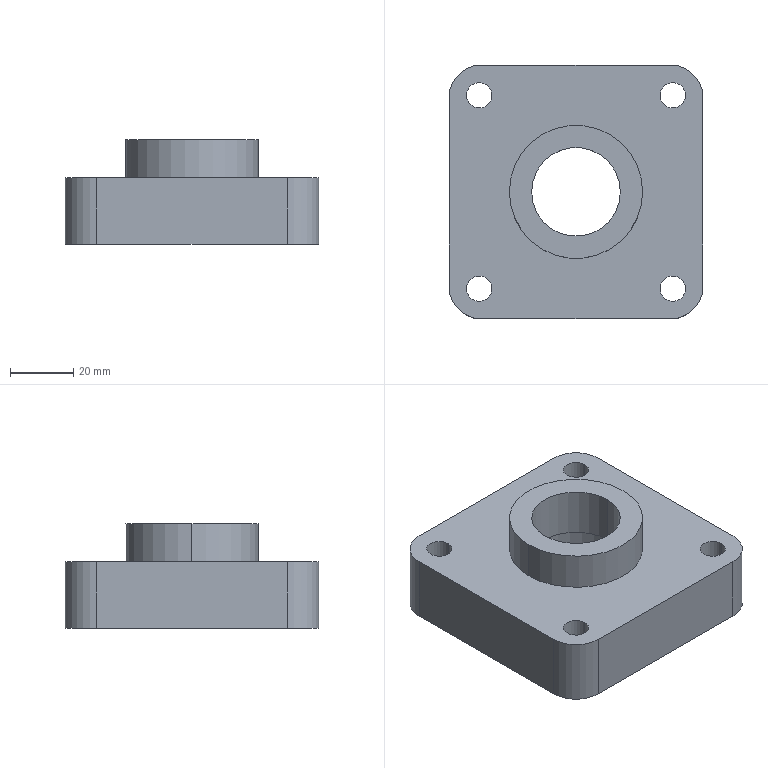Part | SolidWorks | features Fillet 3, ICE 2, MirrorPattern 2, Extrusion 1, RevCut 1 | 1 solid | 39 faces | box 80 x 80 x 33 mm | volume 110292 mm3 | cylinder 24 | plane 11 | torus 4 | commonest cylinder face diameters 8 x8 20 x4 28 x2 35 x2 40 x2 42 x2
STEP:
#1=CARTESIAN_POINT('',(19.,0.,17.5));
#2=VERTEX_POINT('',#1);
#3=CARTESIAN_POINT('',(-19.,0.,17.5));
#4=VERTEX_POINT('',#3);
#5=CARTESIAN_POINT('',(0.,0.,17.5));
#6=DIRECTION('',(0.,0.,-1.));
#7=DIRECTION('',(-1.,0.,0.));
#8=AXIS2_PLACEMENT_3D('',#5,#6,#7);
#9=CIRCLE('',#8,19.);
#10=EDGE_CURVE('',#2,#4,#9,.T.);
#11=ORIENTED_EDGE('',*,*,#10,.F.);
#12=CARTESIAN_POINT('',(20.,0.,16.5));
#13=VERTEX_POINT('',#12);
#14=CARTESIAN_POINT('',(19.,0.,16.5));
#15=DIRECTION('',(0.,1.,0.));
#16=DIRECTION('',(-1.,0.,0.));
#17=AXIS2_PLACEMENT_3D('',#14,#15,#16);
#18=CIRCLE('',#17,1.);
#19=EDGE_CURVE('',#2,#13,#18,.T.);
#20=ORIENTED_EDGE('',*,*,#19,.T.);
#21=CARTESIAN_POINT('',(-20.,0.,16.5));
#22=VERTEX_POINT('',#21);
#23=CARTESIAN_POINT('',(0.,0.,16.5));
#24=DIRECTION('',(0.,0.,1.));
#25=DIRECTION('',(-1.,0.,0.));
#26=AXIS2_PLACEMENT_3D('',#23,#24,#25);
#27=CIRCLE('',#26,20.);
#28=EDGE_CURVE('',#22,#13,#27,.T.);
#29=ORIENTED_EDGE('',*,*,#28,.F.);
#30=CARTESIAN_POINT('',(-19.,0.,16.5));
#31=DIRECTION('',(0.,-1.,0.));
#32=DIRECTION('',(0.,0.,-1.));
#33=AXIS2_PLACEMENT_3D('',#30,#31,#32);
#34=CIRCLE('',#33,1.);
#35=EDGE_CURVE('',#4,#22,#34,.T.);
#36=ORIENTED_EDGE('',*,*,#35,.F.);
#37=EDGE_LOOP('',(#11,#20,#29,#36));
#38=FACE_OUTER_BOUND('',#37,.T.);
#39=CARTESIAN_POINT('',(0.,0.,16.5));
#40=DIRECTION('',(0.,0.,-1.));
#41=DIRECTION('',(-1.,0.,0.));
#42=AXIS2_PLACEMENT_3D('',#39,#40,#41);
#43=TOROIDAL_SURFACE('',#42,19.,1.);
#44=ADVANCED_FACE('',(#38),#43,.F.);
#45=CARTESIAN_POINT('',(29.,0.,2.5));
#46=VERTEX_POINT('',#45);
#47=CARTESIAN_POINT('',(-29.,0.,2.5));
#48=VERTEX_POINT('',#47);
#49=CARTESIAN_POINT('',(0.,0.,2.5));
#50=DIRECTION('',(0.,0.,-1.));
#51=DIRECTION('',(-1.,0.,0.));
#52=AXIS2_PLACEMENT_3D('',#49,#50,#51);
#53=CIRCLE('',#52,29.);
#54=EDGE_CURVE('',#46,#48,#53,.T.);
#55=ORIENTED_EDGE('',*,*,#54,.F.);
#56=CARTESIAN_POINT('',(30.,0.,1.5));
#57=VERTEX_POINT('',#56);
#58=CARTESIAN_POINT('',(29.,0.,1.5));
#59=DIRECTION('',(0.,1.,0.));
#60=DIRECTION('',(-1.,0.,0.));
#61=AXIS2_PLACEMENT_3D('',#58,#59,#60);
#62=CIRCLE('',#61,1.);
#63=EDGE_CURVE('',#46,#57,#62,.T.);
#64=ORIENTED_EDGE('',*,*,#63,.T.);
#65=CARTESIAN_POINT('',(-30.,0.,1.5));
#66=VERTEX_POINT('',#65);
#67=CARTESIAN_POINT('',(0.,0.,1.5));
#68=DIRECTION('',(0.,0.,1.));
#69=DIRECTION('',(-1.,0.,0.));
#70=AXIS2_PLACEMENT_3D('',#67,#68,#69);
#71=CIRCLE('',#70,30.);
#72=EDGE_CURVE('',#66,#57,#71,.T.);
#73=ORIENTED_EDGE('',*,*,#72,.F.);
#74=CARTESIAN_POINT('',(-29.,0.,1.5));
#75=DIRECTION('',(0.,-1.,0.));
#76=DIRECTION('',(0.,0.,-1.));
#77=AXIS2_PLACEMENT_3D('',#74,#75,#76);
#78=CIRCLE('',#77,1.);
#79=EDGE_CURVE('',#48,#66,#78,.T.);
#80=ORIENTED_EDGE('',*,*,#79,.F.);
#81=EDGE_LOOP('',(#55,#64,#73,#80));
#82=FACE_OUTER_BOUND('',#81,.T.);
#83=CARTESIAN_POINT('',(0.,0.,1.5));
#84=DIRECTION('',(0.,0.,-1.));
#85=DIRECTION('',(-1.,0.,0.));
#86=AXIS2_PLACEMENT_3D('',#83,#84,#85);
#87=TOROIDAL_SURFACE('',#86,29.,1.);
#88=ADVANCED_FACE('',(#82),#87,.F.);
#89=CARTESIAN_POINT('',(34.5,30.5,0.));
#90=VERTEX_POINT('',#89);
#91=CARTESIAN_POINT('',(26.5,30.5,0.));
#92=VERTEX_POINT('',#91);
#93=CARTESIAN_POINT('',(30.5,30.5,0.));
#94=DIRECTION('',(0.,0.,-1.));
#95=DIRECTION('',(-1.,0.,0.));
#96=AXIS2_PLACEMENT_3D('',#93,#94,#95);
#97=CIRCLE('',#96,4.);
#98=EDGE_CURVE('',#90,#92,#97,.T.);
#99=ORIENTED_EDGE('',*,*,#98,.T.);
#100=CARTESIAN_POINT('',(26.5,30.5,21.));
#101=VERTEX_POINT('',#100);
#102=CARTESIAN_POINT('',(26.5,30.5,0.));
#103=DIRECTION('',(0.,0.,1.));
#104=VECTOR('',#103,1000.);
#105=LINE('',#102,#104);
#106=EDGE_CURVE('',#92,#101,#105,.T.);
#107=ORIENTED_EDGE('',*,*,#106,.T.);
#108=CARTESIAN_POINT('',(34.5,30.5,21.));
#109=VERTEX_POINT('',#108);
#110=CARTESIAN_POINT('',(30.5,30.5,21.));
#111=DIRECTION('',(0.,0.,-1.));
#112=DIRECTION('',(-1.,0.,0.));
#113=AXIS2_PLACEMENT_3D('',#110,#111,#112);
#114=CIRCLE('',#113,4.);
#115=EDGE_CURVE('',#109,#101,#114,.T.);
#116=ORIENTED_EDGE('',*,*,#115,.F.);
#117=CARTESIAN_POINT('',(34.5,30.5,0.));
#118=DIRECTION('',(0.,0.,1.));
#119=VECTOR('',#118,1000.);
#120=LINE('',#117,#119);
#121=EDGE_CURVE('',#90,#109,#120,.T.);
#122=ORIENTED_EDGE('',*,*,#121,.F.);
#123=EDGE_LOOP('',(#99,#107,#116,#122));
#124=FACE_OUTER_BOUND('',#123,.T.);
#125=CARTESIAN_POINT('',(30.5,30.5,0.));
#126=DIRECTION('',(0.,0.,1.));
#127=DIRECTION('',(1.,0.,0.));
#128=AXIS2_PLACEMENT_3D('',#125,#126,#127);
#129=CYLINDRICAL_SURFACE('',#128,4.);
#130=ADVANCED_FACE('',(#124),#129,.F.);
#131=CARTESIAN_POINT('',(26.5,-30.5,0.));
#132=VERTEX_POINT('',#131);
#133=CARTESIAN_POINT('',(34.5,-30.5,0.));
#134=VERTEX_POINT('',#133);
#135=CARTESIAN_POINT('',(30.5,-30.5,0.));
#136=DIRECTION('',(0.,0.,1.));
#137=DIRECTION('',(-1.,0.,0.));
#138=AXIS2_PLACEMENT_3D('',#135,#136,#137);
#139=CIRCLE('',#138,4.);
#140=EDGE_CURVE('',#132,#134,#139,.T.);
#141=ORIENTED_EDGE('',*,*,#140,.F.);
#142=CARTESIAN_POINT('',(26.5,-30.5,21.));
#143=VERTEX_POINT('',#142);
#144=CARTESIAN_POINT('',(26.5,-30.5,0.));
#145=DIRECTION('',(0.,0.,1.));
#146=VECTOR('',#145,1000.);
#147=LINE('',#144,#146);
#148=EDGE_CURVE('',#132,#143,#147,.T.);
#149=ORIENTED_EDGE('',*,*,#148,.T.);
#150=CARTESIAN_POINT('',(34.5,-30.5,21.));
#151=VERTEX_POINT('',#150);
#152=CARTESIAN_POINT('',(30.5,-30.5,21.));
#153=DIRECTION('',(0.,0.,1.));
#154=DIRECTION('',(-1.,0.,0.));
#155=AXIS2_PLACEMENT_3D('',#152,#153,#154);
#156=CIRCLE('',#155,4.);
#157=EDGE_CURVE('',#143,#151,#156,.T.);
#158=ORIENTED_EDGE('',*,*,#157,.T.);
#159=CARTESIAN_POINT('',(34.5,-30.5,0.));
#160=DIRECTION('',(0.,0.,1.));
#161=VECTOR('',#160,1000.);
#162=LINE('',#159,#161);
#163=EDGE_CURVE('',#134,#151,#162,.T.);
#164=ORIENTED_EDGE('',*,*,#163,.F.);
#165=EDGE_LOOP('',(#141,#149,#158,#164));
#166=FACE_OUTER_BOUND('',#165,.T.);
#167=CARTESIAN_POINT('',(30.5,-30.5,0.));
#168=DIRECTION('',(0.,0.,1.));
#169=DIRECTION('',(1.,0.,0.));
#170=AXIS2_PLACEMENT_3D('',#167,#168,#169);
#171=CYLINDRICAL_SURFACE('',#170,4.);
#172=ADVANCED_FACE('',(#166),#171,.F.);
#173=CARTESIAN_POINT('',(-26.5,-30.5,0.));
#174=VERTEX_POINT('',#173);
#175=CARTESIAN_POINT('',(-34.5,-30.5,0.));
#176=VERTEX_POINT('',#175);
#177=CARTESIAN_POINT('',(-30.5,-30.5,0.));
#178=DIRECTION('',(0.,0.,-1.));
#179=DIRECTION('',(1.,0.,0.));
#180=AXIS2_PLACEMENT_3D('',#177,#178,#179);
#181=CIRCLE('',#180,4.);
#182=EDGE_CURVE('',#174,#176,#181,.T.);
#183=ORIENTED_EDGE('',*,*,#182,.T.);
#184=CARTESIAN_POINT('',(-34.5,-30.5,21.));
#185=VERTEX_POINT('',#184);
#186=CARTESIAN_POINT('',(-34.5,-30.5,0.));
#187=DIRECTION('',(0.,0.,1.));
#188=VECTOR('',#187,1000.);
#189=LINE('',#186,#188);
#190=EDGE_CURVE('',#176,#185,#189,.T.);
#191=ORIENTED_EDGE('',*,*,#190,.T.);
#192=CARTESIAN_POINT('',(-26.5,-30.5,21.));
#193=VERTEX_POINT('',#192);
#194=CARTESIAN_POINT('',(-30.5,-30.5,21.));
#195=DIRECTION('',(0.,0.,-1.));
#196=DIRECTION('',(1.,0.,0.));
#197=AXIS2_PLACEMENT_3D('',#194,#195,#196);
#198=CIRCLE('',#197,4.);
#199=EDGE_CURVE('',#193,#185,#198,.T.);
#200=ORIENTED_EDGE('',*,*,#199,.F.);
#201=CARTESIAN_POINT('',(-26.5,-30.5,0.));
#202=DIRECTION('',(0.,0.,1.));
#203=VECTOR('',#202,1000.);
#204=LINE('',#201,#203);
#205=EDGE_CURVE('',#174,#193,#204,.T.);
#206=ORIENTED_EDGE('',*,*,#205,.F.);
#207=EDGE_LOOP('',(#183,#191,#200,#206));
#208=FACE_OUTER_BOUND('',#207,.T.);
#209=CARTESIAN_POINT('',(-30.5,-30.5,0.));
#210=DIRECTION('',(0.,0.,1.));
#211=DIRECTION('',(1.,0.,0.));
#212=AXIS2_PLACEMENT_3D('',#209,#210,#211);
#213=CYLINDRICAL_SURFACE('',#212,4.);
#214=ADVANCED_FACE('',(#208),#213,.F.);
#215=CARTESIAN_POINT('',(-34.5,30.5,0.));
#216=VERTEX_POINT('',#215);
#217=CARTESIAN_POINT('',(-26.5,30.5,0.));
#218=VERTEX_POINT('',#217);
#219=CARTESIAN_POINT('',(-30.5,30.5,0.));
#220=DIRECTION('',(0.,0.,1.));
#221=DIRECTION('',(1.,0.,0.));
#222=AXIS2_PLACEMENT_3D('',#219,#220,#221);
#223=CIRCLE('',#222,4.);
#224=EDGE_CURVE('',#216,#218,#223,.T.);
#225=ORIENTED_EDGE('',*,*,#224,.F.);
#226=CARTESIAN_POINT('',(-34.5,30.5,21.));
#227=VERTEX_POINT('',#226);
#228=CARTESIAN_POINT('',(-34.5,30.5,0.));
#229=DIRECTION('',(0.,0.,1.));
#230=VECTOR('',#229,1000.);
#231=LINE('',#228,#230);
#232=EDGE_CURVE('',#216,#227,#231,.T.);
#233=ORIENTED_EDGE('',*,*,#232,.T.);
#234=CARTESIAN_POINT('',(-26.5,30.5,21.));
#235=VERTEX_POINT('',#234);
#236=CARTESIAN_POINT('',(-30.5,30.5,21.));
#237=DIRECTION('',(0.,0.,1.));
#238=DIRECTION('',(1.,0.,0.));
#239=AXIS2_PLACEMENT_3D('',#236,#237,#238);
#240=CIRCLE('',#239,4.);
#241=EDGE_CURVE('',#227,#235,#240,.T.);
#242=ORIENTED_EDGE('',*,*,#241,.T.);
#243=CARTESIAN_POINT('',(-26.5,30.5,0.));
#244=DIRECTION('',(0.,0.,1.));
#245=VECTOR('',#244,1000.);
#246=LINE('',#243,#245);
#247=EDGE_CURVE('',#218,#235,#246,.T.);
#248=ORIENTED_EDGE('',*,*,#247,.F.);
#249=EDGE_LOOP('',(#225,#233,#242,#248));
#250=FACE_OUTER_BOUND('',#249,.T.);
#251=CARTESIAN_POINT('',(-30.5,30.5,0.));
#252=DIRECTION('',(0.,0.,1.));
#253=DIRECTION('',(1.,0.,0.));
#254=AXIS2_PLACEMENT_3D('',#251,#252,#253);
#255=CYLINDRICAL_SURFACE('',#254,4.);
#256=ADVANCED_FACE('',(#250),#255,.F.);
#257=ORIENTED_EDGE('',*,*,#72,.T.);
#258=CARTESIAN_POINT('',(30.,0.,0.));
#259=VERTEX_POINT('',#258);
#260=CARTESIAN_POINT('',(30.,0.,0.));
#261=DIRECTION('',(0.,0.,-1.));
#262=VECTOR('',#261,1000.);
#263=LINE('',#260,#262);
#264=EDGE_CURVE('',#57,#259,#263,.T.);
#265=ORIENTED_EDGE('',*,*,#264,.T.);
#266=CARTESIAN_POINT('',(-30.,0.,0.));
#267=VERTEX_POINT('',#266);
#268=CARTESIAN_POINT('',(0.,0.,0.));
#269=DIRECTION('',(0.,0.,-1.));
#270=DIRECTION('',(-1.,0.,0.));
#271=AXIS2_PLACEMENT_3D('',#268,#269,#270);
#272=CIRCLE('',#271,30.);
#273=EDGE_CURVE('',#259,#267,#272,.T.);
#274=ORIENTED_EDGE('',*,*,#273,.T.);
#275=CARTESIAN_POINT('',(-30.,0.,0.));
#276=DIRECTION('',(0.,0.,-1.));
#277=VECTOR('',#276,1000.);
#278=LINE('',#275,#277);
#279=EDGE_CURVE('',#66,#267,#278,.T.);
#280=ORIENTED_EDGE('',*,*,#279,.F.);
#281=EDGE_LOOP('',(#257,#265,#274,#280));
#282=FACE_OUTER_BOUND('',#281,.T.);
#283=CARTESIAN_POINT('',(0.,0.,0.));
#284=DIRECTION('',(0.,0.,-1.));
#285=DIRECTION('',(-1.,0.,0.));
#286=AXIS2_PLACEMENT_3D('',#283,#284,#285);
#287=CYLINDRICAL_SURFACE('',#286,30.);
#288=ADVANCED_FACE('',(#282),#287,.F.);
#289=CARTESIAN_POINT('',(22.5,0.,7.5));
#290=VERTEX_POINT('',#289);
#291=CARTESIAN_POINT('',(-22.5,0.,7.5));
#292=VERTEX_POINT('',#291);
#293=CARTESIAN_POINT('',(0.,0.,7.5));
#294=DIRECTION('',(0.,0.,-1.));
#295=DIRECTION('',(-1.,0.,0.));
#296=AXIS2_PLACEMENT_3D('',#293,#294,#295);
#297=CIRCLE('',#296,22.5);
#298=EDGE_CURVE('',#290,#292,#297,.T.);
#299=ORIENTED_EDGE('',*,*,#298,.F.);
#300=CARTESIAN_POINT('',(22.5,0.,2.5));
#301=VERTEX_POINT('',#300);
#302=CARTESIAN_POINT('',(22.5,0.,0.));
#303=DIRECTION('',(0.,0.,-1.));
#304=VECTOR('',#303,1000.);
#305=LINE('',#302,#304);
#306=EDGE_CURVE('',#290,#301,#305,.T.);
#307=ORIENTED_EDGE('',*,*,#306,.T.);
#308=CARTESIAN_POINT('',(-22.5,0.,2.5));
#309=VERTEX_POINT('',#308);
#310=CARTESIAN_POINT('',(0.,0.,2.5));
#311=DIRECTION('',(0.,0.,-1.));
#312=DIRECTION('',(-1.,0.,0.));
#313=AXIS2_PLACEMENT_3D('',#310,#311,#312);
#314=CIRCLE('',#313,22.5);
#315=EDGE_CURVE('',#301,#309,#314,.T.);
#316=ORIENTED_EDGE('',*,*,#315,.T.);
#317=CARTESIAN_POINT('',(-22.5,0.,0.));
#318=DIRECTION('',(0.,0.,-1.));
#319=VECTOR('',#318,1000.);
#320=LINE('',#317,#319);
#321=EDGE_CURVE('',#292,#309,#320,.T.);
#322=ORIENTED_EDGE('',*,*,#321,.F.);
#323=EDGE_LOOP('',(#299,#307,#316,#322));
#324=FACE_OUTER_BOUND('',#323,.T.);
#325=CARTESIAN_POINT('',(0.,0.,0.));
#326=DIRECTION('',(0.,0.,-1.));
#327=DIRECTION('',(-1.,0.,0.));
#328=AXIS2_PLACEMENT_3D('',#325,#326,#327);
#329=CYLINDRICAL_SURFACE('',#328,22.5);
#330=ADVANCED_FACE('',(#324),#329,.F.);
#331=CARTESIAN_POINT('',(17.5,0.,15.5));
#332=VERTEX_POINT('',#331);
#333=CARTESIAN_POINT('',(-17.5,0.,15.5));
#334=VERTEX_POINT('',#333);
#335=CARTESIAN_POINT('',(0.,0.,15.5));
#336=DIRECTION('',(0.,0.,-1.));
#337=DIRECTION('',(-1.,0.,0.));
#338=AXIS2_PLACEMENT_3D('',#335,#336,#337);
#339=CIRCLE('',#338,17.5);
#340=EDGE_CURVE('',#332,#334,#339,.T.);
#341=ORIENTED_EDGE('',*,*,#340,.F.);
#342=CARTESIAN_POINT('',(17.5,0.,7.5));
#343=VERTEX_POINT('',#342);
#344=CARTESIAN_POINT('',(17.5,0.,0.));
#345=DIRECTION('',(0.,0.,-1.));
#346=VECTOR('',#345,1000.);
#347=LINE('',#344,#346);
#348=EDGE_CURVE('',#332,#343,#347,.T.);
#349=ORIENTED_EDGE('',*,*,#348,.T.);
#350=CARTESIAN_POINT('',(-17.5,0.,7.5));
#351=VERTEX_POINT('',#350);
#352=CARTESIAN_POINT('',(0.,0.,7.5));
#353=DIRECTION('',(0.,0.,-1.));
#354=DIRECTION('',(-1.,0.,0.));
#355=AXIS2_PLACEMENT_3D('',#352,#353,#354);
#356=CIRCLE('',#355,17.5);
#357=EDGE_CURVE('',#343,#351,#356,.T.);
#358=ORIENTED_EDGE('',*,*,#357,.T.);
#359=CARTESIAN_POINT('',(-17.5,0.,0.));
#360=DIRECTION('',(0.,0.,-1.));
#361=VECTOR('',#360,1000.);
#362=LINE('',#359,#361);
#363=EDGE_CURVE('',#334,#351,#362,.T.);
#364=ORIENTED_EDGE('',*,*,#363,.F.);
#365=EDGE_LOOP('',(#341,#349,#358,#364));
#366=FACE_OUTER_BOUND('',#365,.T.);
#367=CARTESIAN_POINT('',(0.,0.,0.));
#368=DIRECTION('',(0.,0.,-1.));
#369=DIRECTION('',(-1.,0.,0.));
#370=AXIS2_PLACEMENT_3D('',#367,#368,#369);
#371=CYLINDRICAL_SURFACE('',#370,17.5);
#372=ADVANCED_FACE('',(#366),#371,.F.);
#373=ORIENTED_EDGE('',*,*,#28,.T.);
#374=CARTESIAN_POINT('',(20.,0.,15.5));
#375=VERTEX_POINT('',#374);
#376=CARTESIAN_POINT('',(20.,0.,0.));
#377=DIRECTION('',(0.,0.,-1.));
#378=VECTOR('',#377,1000.);
#379=LINE('',#376,#378);
#380=EDGE_CURVE('',#13,#375,#379,.T.);
#381=ORIENTED_EDGE('',*,*,#380,.T.);
#382=CARTESIAN_POINT('',(-20.,0.,15.5));
#383=VERTEX_POINT('',#382);
#384=CARTESIAN_POINT('',(0.,0.,15.5));
#385=DIRECTION('',(0.,0.,-1.));
#386=DIRECTION('',(-1.,0.,0.));
#387=AXIS2_PLACEMENT_3D('',#384,#385,#386);
#388=CIRCLE('',#387,20.);
#389=EDGE_CURVE('',#375,#383,#388,.T.);
#390=ORIENTED_EDGE('',*,*,#389,.T.);
#391=CARTESIAN_POINT('',(-20.,0.,0.));
#392=DIRECTION('',(0.,0.,-1.));
#393=VECTOR('',#392,1000.);
#394=LINE('',#391,#393);
#395=EDGE_CURVE('',#22,#383,#394,.T.);
#396=ORIENTED_EDGE('',*,*,#395,.F.);
#397=EDGE_LOOP('',(#373,#381,#390,#396));
#398=FACE_OUTER_BOUND('',#397,.T.);
#399=CARTESIAN_POINT('',(0.,0.,0.));
#400=DIRECTION('',(0.,0.,-1.));
#401=DIRECTION('',(-1.,0.,0.));
#402=AXIS2_PLACEMENT_3D('',#399,#400,#401);
#403=CYLINDRICAL_SURFACE('',#402,20.);
#404=ADVANCED_FACE('',(#398),#403,.F.);
#405=CARTESIAN_POINT('',(14.,0.,33.));
#406=VERTEX_POINT('',#405);
#407=CARTESIAN_POINT('',(-14.,0.,33.));
#408=VERTEX_POINT('',#407);
#409=CARTESIAN_POINT('',(0.,0.,33.));
#410=DIRECTION('',(0.,0.,-1.));
#411=DIRECTION('',(-1.,0.,0.));
#412=AXIS2_PLACEMENT_3D('',#409,#410,#411);
#413=CIRCLE('',#412,14.);
#414=EDGE_CURVE('',#406,#408,#413,.T.);
#415=ORIENTED_EDGE('',*,*,#414,.F.);
#416=CARTESIAN_POINT('',(14.,0.,17.5));
#417=VERTEX_POINT('',#416);
#418=CARTESIAN_POINT('',(14.,0.,0.));
#419=DIRECTION('',(0.,0.,-1.));
#420=VECTOR('',#419,1000.);
#421=LINE('',#418,#420);
#422=EDGE_CURVE('',#406,#417,#421,.T.);
#423=ORIENTED_EDGE('',*,*,#422,.T.);
#424=CARTESIAN_POINT('',(-14.,0.,17.5));
#425=VERTEX_POINT('',#424);
#426=CARTESIAN_POINT('',(0.,0.,17.5));
#427=DIRECTION('',(0.,0.,-1.));
#428=DIRECTION('',(-1.,0.,0.));
#429=AXIS2_PLACEMENT_3D('',#426,#427,#428);
#430=CIRCLE('',#429,14.);
#431=EDGE_CURVE('',#417,#425,#430,.T.);
#432=ORIENTED_EDGE('',*,*,#431,.T.);
#433=CARTESIAN_POINT('',(-14.,0.,0.));
#434=DIRECTION('',(0.,0.,-1.));
#435=VECTOR('',#434,1000.);
#436=LINE('',#433,#435);
#437=EDGE_CURVE('',#408,#425,#436,.T.);
#438=ORIENTED_EDGE('',*,*,#437,.F.);
#439=EDGE_LOOP('',(#415,#423,#432,#438));
#440=FACE_OUTER_BOUND('',#439,.T.);
#441=CARTESIAN_POINT('',(0.,0.,0.));
#442=DIRECTION('',(0.,0.,-1.));
#443=DIRECTION('',(-1.,0.,0.));
#444=AXIS2_PLACEMENT_3D('',#441,#442,#443);
#445=CYLINDRICAL_SURFACE('',#444,14.);
#446=ADVANCED_FACE('',(#440),#445,.F.);
#447=CARTESIAN_POINT('',(21.,0.,33.));
#448=VERTEX_POINT('',#447);
#449=CARTESIAN_POINT('',(-21.,0.,33.));
#450=VERTEX_POINT('',#449);
#451=CARTESIAN_POINT('',(0.,0.,33.));
#452=DIRECTION('',(0.,0.,1.));
#453=DIRECTION('',(1.,0.,0.));
#454=AXIS2_PLACEMENT_3D('',#451,#452,#453);
#455=CIRCLE('',#454,21.);
#456=EDGE_CURVE('',#448,#450,#455,.T.);
#457=ORIENTED_EDGE('',*,*,#456,.F.);
#458=CARTESIAN_POINT('',(21.,0.,21.));
#459=VERTEX_POINT('',#458);
#460=CARTESIAN_POINT('',(21.,0.,33.));
#461=DIRECTION('',(0.,0.,-1.));
#462=VECTOR('',#461,1000.);
#463=LINE('',#460,#462);
#464=EDGE_CURVE('',#448,#459,#463,.T.);
#465=ORIENTED_EDGE('',*,*,#464,.T.);
#466=CARTESIAN_POINT('',(-21.,0.,21.));
#467=VERTEX_POINT('',#466);
#468=CARTESIAN_POINT('',(0.,0.,21.));
#469=DIRECTION('',(0.,0.,1.));
#470=DIRECTION('',(1.,0.,0.));
#471=AXIS2_PLACEMENT_3D('',#468,#469,#470);
#472=CIRCLE('',#471,21.);
#473=EDGE_CURVE('',#459,#467,#472,.T.);
#474=ORIENTED_EDGE('',*,*,#473,.T.);
#475=CARTESIAN_POINT('',(-21.,0.,33.));
#476=DIRECTION('',(0.,0.,-1.));
#477=VECTOR('',#476,1000.);
#478=LINE('',#475,#477);
#479=EDGE_CURVE('',#450,#467,#478,.T.);
#480=ORIENTED_EDGE('',*,*,#479,.F.);
#481=EDGE_LOOP('',(#457,#465,#474,#480));
#482=FACE_OUTER_BOUND('',#481,.T.);
#483=CARTESIAN_POINT('',(0.,0.,33.));
#484=DIRECTION('',(0.,0.,-1.));
#485=DIRECTION('',(-1.,0.,0.));
#486=AXIS2_PLACEMENT_3D('',#483,#484,#485);
#487=CYLINDRICAL_SURFACE('',#486,21.);
#488=ADVANCED_FACE('',(#482),#487,.T.);
#489=CARTESIAN_POINT('',(40.,-30.,21.));
#490=VERTEX_POINT('',#489);
#491=CARTESIAN_POINT('',(40.,30.,21.));
#492=VERTEX_POINT('',#491);
#493=CARTESIAN_POINT('',(40.,-40.,21.));
#494=DIRECTION('',(0.,1.,0.));
#495=VECTOR('',#494,1000.);
#496=LINE('',#493,#495);
#497=EDGE_CURVE('',#490,#492,#496,.T.);
#498=ORIENTED_EDGE('',*,*,#497,.F.);
#499=CARTESIAN_POINT('',(40.,-30.,0.));
#500=VERTEX_POINT('',#499);
#501=CARTESIAN_POINT('',(40.,-30.,21.));
#502=DIRECTION('',(0.,0.,-1.));
#503=VECTOR('',#502,1000.);
#504=LINE('',#501,#503);
#505=EDGE_CURVE('',#490,#500,#504,.T.);
#506=ORIENTED_EDGE('',*,*,#505,.T.);
#507=CARTESIAN_POINT('',(40.,30.,0.));
#508=VERTEX_POINT('',#507);
#509=CARTESIAN_POINT('',(40.,-40.,0.));
#510=DIRECTION('',(0.,1.,0.));
#511=VECTOR('',#510,1000.);
#512=LINE('',#509,#511);
#513=EDGE_CURVE('',#500,#508,#512,.T.);
#514=ORIENTED_EDGE('',*,*,#513,.T.);
#515=CARTESIAN_POINT('',(40.,30.,21.));
#516=DIRECTION('',(0.,0.,1.));
#517=VECTOR('',#516,1000.);
#518=LINE('',#515,#517);
#519=EDGE_CURVE('',#508,#492,#518,.T.);
#520=ORIENTED_EDGE('',*,*,#519,.T.);
#521=EDGE_LOOP('',(#498,#506,#514,#520));
#522=FACE_OUTER_BOUND('',#521,.T.);
#523=CARTESIAN_POINT('',(40.,-40.,21.));
#524=DIRECTION('',(-1.,0.,0.));
#525=DIRECTION('',(0.,0.,1.));
#526=AXIS2_PLACEMENT_3D('',#523,#524,#525);
#527=PLANE('',#526);
#528=ADVANCED_FACE('',(#522),#527,.F.);
#529=CARTESIAN_POINT('',(30.,40.,21.));
#530=VERTEX_POINT('',#529);
#531=CARTESIAN_POINT('',(-30.,40.,21.));
#532=VERTEX_POINT('',#531);
#533=CARTESIAN_POINT('',(-40.,40.,21.));
#534=DIRECTION('',(-1.,0.,0.));
#535=VECTOR('',#534,1000.);
#536=LINE('',#533,#535);
#537=EDGE_CURVE('',#530,#532,#536,.T.);
#538=ORIENTED_EDGE('',*,*,#537,.F.);
#539=CARTESIAN_POINT('',(30.,40.,0.));
#540=VERTEX_POINT('',#539);
#541=CARTESIAN_POINT('',(30.,40.,21.));
#542=DIRECTION('',(0.,0.,-1.));
#543=VECTOR('',#542,1000.);
#544=LINE('',#541,#543);
#545=EDGE_CURVE('',#530,#540,#544,.T.);
#546=ORIENTED_EDGE('',*,*,#545,.T.);
#547=CARTESIAN_POINT('',(-30.,40.,0.));
#548=VERTEX_POINT('',#547);
#549=CARTESIAN_POINT('',(-40.,40.,0.));
#550=DIRECTION('',(-1.,0.,0.));
#551=VECTOR('',#550,1000.);
#552=LINE('',#549,#551);
#553=EDGE_CURVE('',#540,#548,#552,.T.);
#554=ORIENTED_EDGE('',*,*,#553,.T.);
#555=CARTESIAN_POINT('',(-30.,40.,21.));
#556=DIRECTION('',(0.,0.,1.));
#557=VECTOR('',#556,1000.);
#558=LINE('',#555,#557);
#559=EDGE_CURVE('',#548,#532,#558,.T.);
#560=ORIENTED_EDGE('',*,*,#559,.T.);
#561=EDGE_LOOP('',(#538,#546,#554,#560));
#562=FACE_OUTER_BOUND('',#561,.T.);
#563=CARTESIAN_POINT('',(-40.,40.,21.));
#564=DIRECTION('',(0.,-1.,0.));
#565=DIRECTION('',(0.,0.,-1.));
#566=AXIS2_PLACEMENT_3D('',#563,#564,#565);
#567=PLANE('',#566);
#568=ADVANCED_FACE('',(#562),#567,.F.);
#569=CARTESIAN_POINT('',(-40.,30.,0.));
#570=VERTEX_POINT('',#569);
#571=CARTESIAN_POINT('',(-40.,-30.,0.));
#572=VERTEX_POINT('',#571);
#573=CARTESIAN_POINT('',(-40.,-40.,0.));
#574=DIRECTION('',(0.,-1.,0.));
#575=VECTOR('',#574,1000.);
#576=LINE('',#573,#575);
#577=EDGE_CURVE('',#570,#572,#576,.T.);
#578=ORIENTED_EDGE('',*,*,#577,.T.);
#579=CARTESIAN_POINT('',(-40.,-30.,21.));
#580=VERTEX_POINT('',#579);
#581=CARTESIAN_POINT('',(-40.,-30.,21.));
#582=DIRECTION('',(0.,0.,1.));
#583=VECTOR('',#582,1000.);
#584=LINE('',#581,#583);
#585=EDGE_CURVE('',#572,#580,#584,.T.);
#586=ORIENTED_EDGE('',*,*,#585,.T.);
#587=CARTESIAN_POINT('',(-40.,30.,21.));
#588=VERTEX_POINT('',#587);
#589=CARTESIAN_POINT('',(-40.,-40.,21.));
#590=DIRECTION('',(0.,-1.,0.));
#591=VECTOR('',#590,1000.);
#592=LINE('',#589,#591);
#593=EDGE_CURVE('',#588,#580,#592,.T.);
#594=ORIENTED_EDGE('',*,*,#593,.F.);
#595=CARTESIAN_POINT('',(-40.,30.,21.));
#596=DIRECTION('',(0.,0.,-1.));
#597=VECTOR('',#596,1000.);
#598=LINE('',#595,#597);
#599=EDGE_CURVE('',#588,#570,#598,.T.);
#600=ORIENTED_EDGE('',*,*,#599,.T.);
#601=EDGE_LOOP('',(#578,#586,#594,#600));
#602=FACE_OUTER_BOUND('',#601,.T.);
#603=CARTESIAN_POINT('',(-40.,-40.,21.));
#604=DIRECTION('',(1.,0.,0.));
#605=DIRECTION('',(0.,0.,-1.));
#606=AXIS2_PLACEMENT_3D('',#603,#604,#605);
#607=PLANE('',#606);
#608=ADVANCED_FACE('',(#602),#607,.F.);
#609=CARTESIAN_POINT('',(-30.,-40.,0.));
#610=VERTEX_POINT('',#609);
#611=CARTESIAN_POINT('',(30.,-40.,0.));
#612=VERTEX_POINT('',#611);
#613=CARTESIAN_POINT('',(-40.,-40.,0.));
#614=DIRECTION('',(1.,0.,0.));
#615=VECTOR('',#614,1000.);
#616=LINE('',#613,#615);
#617=EDGE_CURVE('',#610,#612,#616,.T.);
#618=ORIENTED_EDGE('',*,*,#617,.T.);
#619=CARTESIAN_POINT('',(30.,-40.,21.));
#620=VERTEX_POINT('',#619);
#621=CARTESIAN_POINT('',(30.,-40.,21.));
#622=DIRECTION('',(0.,0.,1.));
#623=VECTOR('',#622,1000.);
#624=LINE('',#621,#623);
#625=EDGE_CURVE('',#612,#620,#624,.T.);
#626=ORIENTED_EDGE('',*,*,#625,.T.);
#627=CARTESIAN_POINT('',(-30.,-40.,21.));
#628=VERTEX_POINT('',#627);
#629=CARTESIAN_POINT('',(-40.,-40.,21.));
#630=DIRECTION('',(1.,0.,0.));
#631=VECTOR('',#630,1000.);
#632=LINE('',#629,#631);
#633=EDGE_CURVE('',#628,#620,#632,.T.);
#634=ORIENTED_EDGE('',*,*,#633,.F.);
#635=CARTESIAN_POINT('',(-30.,-40.,21.));
#636=DIRECTION('',(0.,0.,-1.));
#637=VECTOR('',#636,1000.);
#638=LINE('',#635,#637);
#639=EDGE_CURVE('',#628,#610,#638,.T.);
#640=ORIENTED_EDGE('',*,*,#639,.T.);
#641=EDGE_LOOP('',(#618,#626,#634,#640));
#642=FACE_OUTER_BOUND('',#641,.T.);
#643=CARTESIAN_POINT('',(-40.,-40.,21.));
#644=DIRECTION('',(0.,1.,0.));
#645=DIRECTION('',(0.,0.,1.));
#646=AXIS2_PLACEMENT_3D('',#643,#644,#645);
#647=PLANE('',#646);
#648=ADVANCED_FACE('',(#642),#647,.F.);
#649=ORIENTED_EDGE('',*,*,#115,.T.);
#650=CARTESIAN_POINT('',(30.5,30.5,21.));
#651=DIRECTION('',(0.,0.,-1.));
#652=DIRECTION('',(-1.,0.,0.));
#653=AXIS2_PLACEMENT_3D('',#650,#651,#652);
#654=CIRCLE('',#653,4.);
#655=EDGE_CURVE('',#101,#109,#654,.T.);
#656=ORIENTED_EDGE('',*,*,#655,.T.);
#657=EDGE_LOOP('',(#649,#656));
#658=FACE_BOUND('',#657,.T.);
#659=CARTESIAN_POINT('',(30.5,-30.5,21.));
#660=DIRECTION('',(0.,0.,1.));
#661=DIRECTION('',(-1.,0.,0.));
#662=AXIS2_PLACEMENT_3D('',#659,#660,#661);
#663=CIRCLE('',#662,4.);
#664=EDGE_CURVE('',#151,#143,#663,.T.);
#665=ORIENTED_EDGE('',*,*,#664,.F.);
#666=ORIENTED_EDGE('',*,*,#157,.F.);
#667=EDGE_LOOP('',(#665,#666));
#668=FACE_BOUND('',#667,.T.);
#669=ORIENTED_EDGE('',*,*,#199,.T.);
#670=CARTESIAN_POINT('',(-30.5,-30.5,21.));
#671=DIRECTION('',(0.,0.,-1.));
#672=DIRECTION('',(1.,0.,0.));
#673=AXIS2_PLACEMENT_3D('',#670,#671,#672);
#674=CIRCLE('',#673,4.);
#675=EDGE_CURVE('',#185,#193,#674,.T.);
#676=ORIENTED_EDGE('',*,*,#675,.T.);
#677=EDGE_LOOP('',(#669,#676));
#678=FACE_BOUND('',#677,.T.);
#679=CARTESIAN_POINT('',(-30.5,30.5,21.));
#680=DIRECTION('',(0.,0.,1.));
#681=DIRECTION('',(1.,0.,0.));
#682=AXIS2_PLACEMENT_3D('',#679,#680,#681);
#683=CIRCLE('',#682,4.);
#684=EDGE_CURVE('',#235,#227,#683,.T.);
#685=ORIENTED_EDGE('',*,*,#684,.F.);
#686=ORIENTED_EDGE('',*,*,#241,.F.);
#687=EDGE_LOOP('',(#685,#686));
#688=FACE_BOUND('',#687,.T.);
#689=CARTESIAN_POINT('',(0.,0.,21.));
#690=DIRECTION('',(0.,0.,1.));
#691=DIRECTION('',(1.,0.,0.));
#692=AXIS2_PLACEMENT_3D('',#689,#690,#691);
#693=CIRCLE('',#692,21.);
#694=EDGE_CURVE('',#467,#459,#693,.T.);
#695=ORIENTED_EDGE('',*,*,#694,.F.);
#696=ORIENTED_EDGE('',*,*,#473,.F.);
#697=EDGE_LOOP('',(#695,#696));
#698=FACE_BOUND('',#697,.T.);
#699=ORIENTED_EDGE('',*,*,#633,.T.);
#700=CARTESIAN_POINT('',(30.,-30.,21.));
#701=DIRECTION('',(0.,0.,1.));
#702=DIRECTION('',(-1.,0.,0.));
#703=AXIS2_PLACEMENT_3D('',#700,#701,#702);
#704=CIRCLE('',#703,10.);
#705=EDGE_CURVE('',#620,#490,#704,.T.);
#706=ORIENTED_EDGE('',*,*,#705,.T.);
#707=ORIENTED_EDGE('',*,*,#497,.T.);
#708=CARTESIAN_POINT('',(30.,30.,21.));
#709=DIRECTION('',(0.,0.,1.));
#710=DIRECTION('',(-1.,0.,0.));
#711=AXIS2_PLACEMENT_3D('',#708,#709,#710);
#712=CIRCLE('',#711,10.);
#713=EDGE_CURVE('',#492,#530,#712,.T.);
#714=ORIENTED_EDGE('',*,*,#713,.T.);
#715=ORIENTED_EDGE('',*,*,#537,.T.);
#716=CARTESIAN_POINT('',(-30.,30.,21.));
#717=DIRECTION('',(0.,0.,1.));
#718=DIRECTION('',(-1.,0.,0.));
#719=AXIS2_PLACEMENT_3D('',#716,#717,#718);
#720=CIRCLE('',#719,10.);
#721=EDGE_CURVE('',#532,#588,#720,.T.);
#722=ORIENTED_EDGE('',*,*,#721,.T.);
#723=ORIENTED_EDGE('',*,*,#593,.T.);
#724=CARTESIAN_POINT('',(-30.,-30.,21.));
#725=DIRECTION('',(0.,0.,1.));
#726=DIRECTION('',(-1.,0.,0.));
#727=AXIS2_PLACEMENT_3D('',#724,#725,#726);
#728=CIRCLE('',#727,10.);
#729=EDGE_CURVE('',#580,#628,#728,.T.);
#730=ORIENTED_EDGE('',*,*,#729,.T.);
#731=EDGE_LOOP('',(#699,#706,#707,#714,#715,#722,#723,#730));
#732=FACE_OUTER_BOUND('',#731,.T.);
#733=CARTESIAN_POINT('',(0.,0.,21.));
#734=DIRECTION('',(0.,0.,-1.));
#735=DIRECTION('',(-1.,0.,0.));
#736=AXIS2_PLACEMENT_3D('',#733,#734,#735);
#737=PLANE('',#736);
#738=ADVANCED_FACE('',(#658,#668,#678,#688,#698,#732),#737,.F.);
#739=ORIENTED_EDGE('',*,*,#98,.F.);
#740=CARTESIAN_POINT('',(30.5,30.5,0.));
#741=DIRECTION('',(0.,0.,-1.));
#742=DIRECTION('',(-1.,0.,0.));
#743=AXIS2_PLACEMENT_3D('',#740,#741,#742);
#744=CIRCLE('',#743,4.);
#745=EDGE_CURVE('',#92,#90,#744,.T.);
#746=ORIENTED_EDGE('',*,*,#745,.F.);
#747=EDGE_LOOP('',(#739,#746));
#748=FACE_BOUND('',#747,.T.);
#749=CARTESIAN_POINT('',(30.5,-30.5,0.));
#750=DIRECTION('',(0.,0.,1.));
#751=DIRECTION('',(-1.,0.,0.));
#752=AXIS2_PLACEMENT_3D('',#749,#750,#751);
#753=CIRCLE('',#752,4.);
#754=EDGE_CURVE('',#134,#132,#753,.T.);
#755=ORIENTED_EDGE('',*,*,#754,.T.);
#756=ORIENTED_EDGE('',*,*,#140,.T.);
#757=EDGE_LOOP('',(#755,#756));
#758=FACE_BOUND('',#757,.T.);
#759=ORIENTED_EDGE('',*,*,#182,.F.);
#760=CARTESIAN_POINT('',(-30.5,-30.5,0.));
#761=DIRECTION('',(0.,0.,-1.));
#762=DIRECTION('',(1.,0.,0.));
#763=AXIS2_PLACEMENT_3D('',#760,#761,#762);
#764=CIRCLE('',#763,4.);
#765=EDGE_CURVE('',#176,#174,#764,.T.);
#766=ORIENTED_EDGE('',*,*,#765,.F.);
#767=EDGE_LOOP('',(#759,#766));
#768=FACE_BOUND('',#767,.T.);
#769=CARTESIAN_POINT('',(-30.5,30.5,0.));
#770=DIRECTION('',(0.,0.,1.));
#771=DIRECTION('',(1.,0.,0.));
#772=AXIS2_PLACEMENT_3D('',#769,#770,#771);
#773=CIRCLE('',#772,4.);
#774=EDGE_CURVE('',#218,#216,#773,.T.);
#775=ORIENTED_EDGE('',*,*,#774,.T.);
#776=ORIENTED_EDGE('',*,*,#224,.T.);
#777=EDGE_LOOP('',(#775,#776));
#778=FACE_BOUND('',#777,.T.);
#779=CARTESIAN_POINT('',(0.,0.,0.));
#780=DIRECTION('',(0.,0.,-1.));
#781=DIRECTION('',(-1.,0.,0.));
#782=AXIS2_PLACEMENT_3D('',#779,#780,#781);
#783=CIRCLE('',#782,30.);
#784=EDGE_CURVE('',#267,#259,#783,.T.);
#785=ORIENTED_EDGE('',*,*,#784,.F.);
#786=ORIENTED_EDGE('',*,*,#273,.F.);
#787=EDGE_LOOP('',(#785,#786));
#788=FACE_BOUND('',#787,.T.);
#789=ORIENTED_EDGE('',*,*,#513,.F.);
#790=CARTESIAN_POINT('',(30.,-30.,0.));
#791=DIRECTION('',(0.,0.,-1.));
#792=DIRECTION('',(-1.,0.,0.));
#793=AXIS2_PLACEMENT_3D('',#790,#791,#792);
#794=CIRCLE('',#793,10.);
#795=EDGE_CURVE('',#500,#612,#794,.T.);
#796=ORIENTED_EDGE('',*,*,#795,.T.);
#797=ORIENTED_EDGE('',*,*,#617,.F.);
#798=CARTESIAN_POINT('',(-30.,-30.,0.));
#799=DIRECTION('',(0.,0.,-1.));
#800=DIRECTION('',(-1.,0.,0.));
#801=AXIS2_PLACEMENT_3D('',#798,#799,#800);
#802=CIRCLE('',#801,10.);
#803=EDGE_CURVE('',#610,#572,#802,.T.);
#804=ORIENTED_EDGE('',*,*,#803,.T.);
#805=ORIENTED_EDGE('',*,*,#577,.F.);
#806=CARTESIAN_POINT('',(-30.,30.,0.));
#807=DIRECTION('',(0.,0.,-1.));
#808=DIRECTION('',(-1.,0.,0.));
#809=AXIS2_PLACEMENT_3D('',#806,#807,#808);
#810=CIRCLE('',#809,10.);
#811=EDGE_CURVE('',#570,#548,#810,.T.);
#812=ORIENTED_EDGE('',*,*,#811,.T.);
#813=ORIENTED_EDGE('',*,*,#553,.F.);
#814=CARTESIAN_POINT('',(30.,30.,0.));
#815=DIRECTION('',(0.,0.,-1.));
#816=DIRECTION('',(-1.,0.,0.));
#817=AXIS2_PLACEMENT_3D('',#814,#815,#816);
#818=CIRCLE('',#817,10.);
#819=EDGE_CURVE('',#540,#508,#818,.T.);
#820=ORIENTED_EDGE('',*,*,#819,.T.);
#821=EDGE_LOOP('',(#789,#796,#797,#804,#805,#812,#813,#820));
#822=FACE_OUTER_BOUND('',#821,.T.);
#823=CARTESIAN_POINT('',(0.,0.,0.));
#824=DIRECTION('',(0.,0.,-1.));
#825=DIRECTION('',(-1.,0.,0.));
#826=AXIS2_PLACEMENT_3D('',#823,#824,#825);
#827=PLANE('',#826);
#828=ADVANCED_FACE('',(#748,#758,#768,#778,#788,#822),#827,.T.);
#829=ORIENTED_EDGE('',*,*,#464,.F.);
#830=CARTESIAN_POINT('',(0.,0.,33.));
#831=DIRECTION('',(0.,0.,1.));
#832=DIRECTION('',(1.,0.,0.));
#833=AXIS2_PLACEMENT_3D('',#830,#831,#832);
#834=CIRCLE('',#833,21.);
#835=EDGE_CURVE('',#450,#448,#834,.T.);
#836=ORIENTED_EDGE('',*,*,#835,.F.);
#837=ORIENTED_EDGE('',*,*,#479,.T.);
#838=ORIENTED_EDGE('',*,*,#694,.T.);
#839=EDGE_LOOP('',(#829,#836,#837,#838));
#840=FACE_OUTER_BOUND('',#839,.T.);
#841=CARTESIAN_POINT('',(0.,0.,33.));
#842=DIRECTION('',(0.,0.,-1.));
#843=DIRECTION('',(-1.,0.,0.));
#844=AXIS2_PLACEMENT_3D('',#841,#842,#843);
#845=CYLINDRICAL_SURFACE('',#844,21.);
#846=ADVANCED_FACE('',(#840),#845,.T.);
#847=CARTESIAN_POINT('',(0.,0.,33.));
#848=DIRECTION('',(0.,0.,-1.));
#849=DIRECTION('',(-1.,0.,0.));
#850=AXIS2_PLACEMENT_3D('',#847,#848,#849);
#851=CIRCLE('',#850,14.);
#852=EDGE_CURVE('',#408,#406,#851,.T.);
#853=ORIENTED_EDGE('',*,*,#852,.T.);
#854=ORIENTED_EDGE('',*,*,#414,.T.);
#855=EDGE_LOOP('',(#853,#854));
#856=FACE_BOUND('',#855,.T.);
#857=ORIENTED_EDGE('',*,*,#835,.T.);
#858=ORIENTED_EDGE('',*,*,#456,.T.);
#859=EDGE_LOOP('',(#857,#858));
#860=FACE_OUTER_BOUND('',#859,.T.);
#861=CARTESIAN_POINT('',(0.,0.,33.));
#862=DIRECTION('',(0.,0.,1.));
#863=DIRECTION('',(1.,0.,0.));
#864=AXIS2_PLACEMENT_3D('',#861,#862,#863);
#865=PLANE('',#864);
#866=ADVANCED_FACE('',(#856,#860),#865,.T.);
#867=ORIENTED_EDGE('',*,*,#422,.F.);
#868=ORIENTED_EDGE('',*,*,#852,.F.);
#869=ORIENTED_EDGE('',*,*,#437,.T.);
#870=CARTESIAN_POINT('',(0.,0.,17.5));
#871=DIRECTION('',(0.,0.,-1.));
#872=DIRECTION('',(-1.,0.,0.));
#873=AXIS2_PLACEMENT_3D('',#870,#871,#872);
#874=CIRCLE('',#873,14.);
#875=EDGE_CURVE('',#425,#417,#874,.T.);
#876=ORIENTED_EDGE('',*,*,#875,.T.);
#877=EDGE_LOOP('',(#867,#868,#869,#876));
#878=FACE_OUTER_BOUND('',#877,.T.);
#879=CARTESIAN_POINT('',(0.,0.,0.));
#880=DIRECTION('',(0.,0.,-1.));
#881=DIRECTION('',(-1.,0.,0.));
#882=AXIS2_PLACEMENT_3D('',#879,#880,#881);
#883=CYLINDRICAL_SURFACE('',#882,14.);
#884=ADVANCED_FACE('',(#878),#883,.F.);
#885=CARTESIAN_POINT('',(0.,0.,17.5));
#886=DIRECTION('',(0.,0.,-1.));
#887=DIRECTION('',(-1.,0.,0.));
#888=AXIS2_PLACEMENT_3D('',#885,#886,#887);
#889=CIRCLE('',#888,19.);
#890=EDGE_CURVE('',#4,#2,#889,.T.);
#891=ORIENTED_EDGE('',*,*,#890,.T.);
#892=ORIENTED_EDGE('',*,*,#10,.T.);
#893=EDGE_LOOP('',(#891,#892));
#894=FACE_OUTER_BOUND('',#893,.T.);
#895=ORIENTED_EDGE('',*,*,#875,.F.);
#896=ORIENTED_EDGE('',*,*,#431,.F.);
#897=EDGE_LOOP('',(#895,#896));
#898=FACE_BOUND('',#897,.T.);
#899=CARTESIAN_POINT('',(20.,0.,17.5));
#900=DIRECTION('',(0.,0.,-1.));
#901=DIRECTION('',(-1.,0.,0.));
#902=AXIS2_PLACEMENT_3D('',#899,#900,#901);
#903=PLANE('',#902);
#904=ADVANCED_FACE('',(#894,#898),#903,.T.);
#905=ORIENTED_EDGE('',*,*,#380,.F.);
#906=CARTESIAN_POINT('',(0.,0.,16.5));
#907=DIRECTION('',(0.,0.,1.));
#908=DIRECTION('',(-1.,0.,0.));
#909=AXIS2_PLACEMENT_3D('',#906,#907,#908);
#910=CIRCLE('',#909,20.);
#911=EDGE_CURVE('',#13,#22,#910,.T.);
#912=ORIENTED_EDGE('',*,*,#911,.T.);
#913=ORIENTED_EDGE('',*,*,#395,.T.);
#914=CARTESIAN_POINT('',(0.,0.,15.5));
#915=DIRECTION('',(0.,0.,-1.));
#916=DIRECTION('',(-1.,0.,0.));
#917=AXIS2_PLACEMENT_3D('',#914,#915,#916);
#918=CIRCLE('',#917,20.);
#919=EDGE_CURVE('',#383,#375,#918,.T.);
#920=ORIENTED_EDGE('',*,*,#919,.T.);
#921=EDGE_LOOP('',(#905,#912,#913,#920));
#922=FACE_OUTER_BOUND('',#921,.T.);
#923=CARTESIAN_POINT('',(0.,0.,0.));
#924=DIRECTION('',(0.,0.,-1.));
#925=DIRECTION('',(-1.,0.,0.));
#926=AXIS2_PLACEMENT_3D('',#923,#924,#925);
#927=CYLINDRICAL_SURFACE('',#926,20.);
#928=ADVANCED_FACE('',(#922),#927,.F.);
#929=CARTESIAN_POINT('',(0.,0.,15.5));
#930=DIRECTION('',(0.,0.,-1.));
#931=DIRECTION('',(-1.,0.,0.));
#932=AXIS2_PLACEMENT_3D('',#929,#930,#931);
#933=CIRCLE('',#932,17.5);
#934=EDGE_CURVE('',#334,#332,#933,.T.);
#935=ORIENTED_EDGE('',*,*,#934,.T.);
#936=ORIENTED_EDGE('',*,*,#340,.T.);
#937=EDGE_LOOP('',(#935,#936));
#938=FACE_BOUND('',#937,.T.);
#939=ORIENTED_EDGE('',*,*,#919,.F.);
#940=ORIENTED_EDGE('',*,*,#389,.F.);
#941=EDGE_LOOP('',(#939,#940));
#942=FACE_OUTER_BOUND('',#941,.T.);
#943=CARTESIAN_POINT('',(17.5,0.,15.5));
#944=DIRECTION('',(0.,0.,1.));
#945=DIRECTION('',(1.,0.,0.));
#946=AXIS2_PLACEMENT_3D('',#943,#944,#945);
#947=PLANE('',#946);
#948=ADVANCED_FACE('',(#938,#942),#947,.T.);
#949=ORIENTED_EDGE('',*,*,#348,.F.);
#950=ORIENTED_EDGE('',*,*,#934,.F.);
#951=ORIENTED_EDGE('',*,*,#363,.T.);
#952=CARTESIAN_POINT('',(0.,0.,7.5));
#953=DIRECTION('',(0.,0.,-1.));
#954=DIRECTION('',(-1.,0.,0.));
#955=AXIS2_PLACEMENT_3D('',#952,#953,#954);
#956=CIRCLE('',#955,17.5);
#957=EDGE_CURVE('',#351,#343,#956,.T.);
#958=ORIENTED_EDGE('',*,*,#957,.T.);
#959=EDGE_LOOP('',(#949,#950,#951,#958));
#960=FACE_OUTER_BOUND('',#959,.T.);
#961=CARTESIAN_POINT('',(0.,0.,0.));
#962=DIRECTION('',(0.,0.,-1.));
#963=DIRECTION('',(-1.,0.,0.));
#964=AXIS2_PLACEMENT_3D('',#961,#962,#963);
#965=CYLINDRICAL_SURFACE('',#964,17.5);
#966=ADVANCED_FACE('',(#960),#965,.F.);
#967=CARTESIAN_POINT('',(0.,0.,7.5));
#968=DIRECTION('',(0.,0.,-1.));
#969=DIRECTION('',(-1.,0.,0.));
#970=AXIS2_PLACEMENT_3D('',#967,#968,#969);
#971=CIRCLE('',#970,22.5);
#972=EDGE_CURVE('',#292,#290,#971,.T.);
#973=ORIENTED_EDGE('',*,*,#972,.T.);
#974=ORIENTED_EDGE('',*,*,#298,.T.);
#975=EDGE_LOOP('',(#973,#974));
#976=FACE_OUTER_BOUND('',#975,.T.);
#977=ORIENTED_EDGE('',*,*,#957,.F.);
#978=ORIENTED_EDGE('',*,*,#357,.F.);
#979=EDGE_LOOP('',(#977,#978));
#980=FACE_BOUND('',#979,.T.);
#981=CARTESIAN_POINT('',(22.5,0.,7.5));
#982=DIRECTION('',(0.,0.,-1.));
#983=DIRECTION('',(-1.,0.,0.));
#984=AXIS2_PLACEMENT_3D('',#981,#982,#983);
#985=PLANE('',#984);
#986=ADVANCED_FACE('',(#976,#980),#985,.T.);
#987=ORIENTED_EDGE('',*,*,#306,.F.);
#988=ORIENTED_EDGE('',*,*,#972,.F.);
#989=ORIENTED_EDGE('',*,*,#321,.T.);
#990=CARTESIAN_POINT('',(0.,0.,2.5));
#991=DIRECTION('',(0.,0.,-1.));
#992=DIRECTION('',(-1.,0.,0.));
#993=AXIS2_PLACEMENT_3D('',#990,#991,#992);
#994=CIRCLE('',#993,22.5);
#995=EDGE_CURVE('',#309,#301,#994,.T.);
#996=ORIENTED_EDGE('',*,*,#995,.T.);
#997=EDGE_LOOP('',(#987,#988,#989,#996));
#998=FACE_OUTER_BOUND('',#997,.T.);
#999=CARTESIAN_POINT('',(0.,0.,0.));
#1000=DIRECTION('',(0.,0.,-1.));
#1001=DIRECTION('',(-1.,0.,0.));
#1002=AXIS2_PLACEMENT_3D('',#999,#1000,#1001);
#1003=CYLINDRICAL_SURFACE('',#1002,22.5);
#1004=ADVANCED_FACE('',(#998),#1003,.F.);
#1005=CARTESIAN_POINT('',(0.,0.,2.5));
#1006=DIRECTION('',(0.,0.,-1.));
#1007=DIRECTION('',(-1.,0.,0.));
#1008=AXIS2_PLACEMENT_3D('',#1005,#1006,#1007);
#1009=CIRCLE('',#1008,29.);
#1010=EDGE_CURVE('',#48,#46,#1009,.T.);
#1011=ORIENTED_EDGE('',*,*,#1010,.T.);
#1012=ORIENTED_EDGE('',*,*,#54,.T.);
#1013=EDGE_LOOP('',(#1011,#1012));
#1014=FACE_OUTER_BOUND('',#1013,.T.);
#1015=ORIENTED_EDGE('',*,*,#995,.F.);
#1016=ORIENTED_EDGE('',*,*,#315,.F.);
#1017=EDGE_LOOP('',(#1015,#1016));
#1018=FACE_BOUND('',#1017,.T.);
#1019=CARTESIAN_POINT('',(30.,0.,2.5));
#1020=DIRECTION('',(0.,0.,-1.));
#1021=DIRECTION('',(-1.,0.,0.));
#1022=AXIS2_PLACEMENT_3D('',#1019,#1020,#1021);
#1023=PLANE('',#1022);
#1024=ADVANCED_FACE('',(#1014,#1018),#1023,.T.);
#1025=ORIENTED_EDGE('',*,*,#264,.F.);
#1026=CARTESIAN_POINT('',(0.,0.,1.5));
#1027=DIRECTION('',(0.,0.,1.));
#1028=DIRECTION('',(-1.,0.,0.));
#1029=AXIS2_PLACEMENT_3D('',#1026,#1027,#1028);
#1030=CIRCLE('',#1029,30.);
#1031=EDGE_CURVE('',#57,#66,#1030,.T.);
#1032=ORIENTED_EDGE('',*,*,#1031,.T.);
#1033=ORIENTED_EDGE('',*,*,#279,.T.);
#1034=ORIENTED_EDGE('',*,*,#784,.T.);
#1035=EDGE_LOOP('',(#1025,#1032,#1033,#1034));
#1036=FACE_OUTER_BOUND('',#1035,.T.);
#1037=CARTESIAN_POINT('',(0.,0.,0.));
#1038=DIRECTION('',(0.,0.,-1.));
#1039=DIRECTION('',(-1.,0.,0.));
#1040=AXIS2_PLACEMENT_3D('',#1037,#1038,#1039);
#1041=CYLINDRICAL_SURFACE('',#1040,30.);
#1042=ADVANCED_FACE('',(#1036),#1041,.F.);
#1043=ORIENTED_EDGE('',*,*,#705,.F.);
#1044=ORIENTED_EDGE('',*,*,#625,.F.);
#1045=ORIENTED_EDGE('',*,*,#795,.F.);
#1046=ORIENTED_EDGE('',*,*,#505,.F.);
#1047=EDGE_LOOP('',(#1043,#1044,#1045,#1046));
#1048=FACE_OUTER_BOUND('',#1047,.T.);
#1049=CARTESIAN_POINT('',(30.,-30.,21.));
#1050=DIRECTION('',(0.,0.,-1.));
#1051=DIRECTION('',(-1.,0.,0.));
#1052=AXIS2_PLACEMENT_3D('',#1049,#1050,#1051);
#1053=CYLINDRICAL_SURFACE('',#1052,10.);
#1054=ADVANCED_FACE('',(#1048),#1053,.T.);
#1055=ORIENTED_EDGE('',*,*,#729,.F.);
#1056=ORIENTED_EDGE('',*,*,#585,.F.);
#1057=ORIENTED_EDGE('',*,*,#803,.F.);
#1058=ORIENTED_EDGE('',*,*,#639,.F.);
#1059=EDGE_LOOP('',(#1055,#1056,#1057,#1058));
#1060=FACE_OUTER_BOUND('',#1059,.T.);
#1061=CARTESIAN_POINT('',(-30.,-30.,21.));
#1062=DIRECTION('',(0.,0.,-1.));
#1063=DIRECTION('',(-1.,0.,0.));
#1064=AXIS2_PLACEMENT_3D('',#1061,#1062,#1063);
#1065=CYLINDRICAL_SURFACE('',#1064,10.);
#1066=ADVANCED_FACE('',(#1060),#1065,.T.);
#1067=ORIENTED_EDGE('',*,*,#713,.F.);
#1068=ORIENTED_EDGE('',*,*,#519,.F.);
#1069=ORIENTED_EDGE('',*,*,#819,.F.);
#1070=ORIENTED_EDGE('',*,*,#545,.F.);
#1071=EDGE_LOOP('',(#1067,#1068,#1069,#1070));
#1072=FACE_OUTER_BOUND('',#1071,.T.);
#1073=CARTESIAN_POINT('',(30.,30.,21.));
#1074=DIRECTION('',(0.,0.,-1.));
#1075=DIRECTION('',(-1.,0.,0.));
#1076=AXIS2_PLACEMENT_3D('',#1073,#1074,#1075);
#1077=CYLINDRICAL_SURFACE('',#1076,10.);
#1078=ADVANCED_FACE('',(#1072),#1077,.T.);
#1079=ORIENTED_EDGE('',*,*,#721,.F.);
#1080=ORIENTED_EDGE('',*,*,#559,.F.);
#1081=ORIENTED_EDGE('',*,*,#811,.F.);
#1082=ORIENTED_EDGE('',*,*,#599,.F.);
#1083=EDGE_LOOP('',(#1079,#1080,#1081,#1082));
#1084=FACE_OUTER_BOUND('',#1083,.T.);
#1085=CARTESIAN_POINT('',(-30.,30.,21.));
#1086=DIRECTION('',(0.,0.,-1.));
#1087=DIRECTION('',(-1.,0.,0.));
#1088=AXIS2_PLACEMENT_3D('',#1085,#1086,#1087);
#1089=CYLINDRICAL_SURFACE('',#1088,10.);
#1090=ADVANCED_FACE('',(#1084),#1089,.T.);
#1091=ORIENTED_EDGE('',*,*,#232,.F.);
#1092=ORIENTED_EDGE('',*,*,#774,.F.);
#1093=ORIENTED_EDGE('',*,*,#247,.T.);
#1094=ORIENTED_EDGE('',*,*,#684,.T.);
#1095=EDGE_LOOP('',(#1091,#1092,#1093,#1094));
#1096=FACE_OUTER_BOUND('',#1095,.T.);
#1097=CARTESIAN_POINT('',(-30.5,30.5,0.));
#1098=DIRECTION('',(0.,0.,1.));
#1099=DIRECTION('',(1.,0.,0.));
#1100=AXIS2_PLACEMENT_3D('',#1097,#1098,#1099);
#1101=CYLINDRICAL_SURFACE('',#1100,4.);
#1102=ADVANCED_FACE('',(#1096),#1101,.F.);
#1103=ORIENTED_EDGE('',*,*,#190,.F.);
#1104=ORIENTED_EDGE('',*,*,#765,.T.);
#1105=ORIENTED_EDGE('',*,*,#205,.T.);
#1106=ORIENTED_EDGE('',*,*,#675,.F.);
#1107=EDGE_LOOP('',(#1103,#1104,#1105,#1106));
#1108=FACE_OUTER_BOUND('',#1107,.T.);
#1109=CARTESIAN_POINT('',(-30.5,-30.5,0.));
#1110=DIRECTION('',(0.,0.,1.));
#1111=DIRECTION('',(1.,0.,0.));
#1112=AXIS2_PLACEMENT_3D('',#1109,#1110,#1111);
#1113=CYLINDRICAL_SURFACE('',#1112,4.);
#1114=ADVANCED_FACE('',(#1108),#1113,.F.);
#1115=ORIENTED_EDGE('',*,*,#148,.F.);
#1116=ORIENTED_EDGE('',*,*,#754,.F.);
#1117=ORIENTED_EDGE('',*,*,#163,.T.);
#1118=ORIENTED_EDGE('',*,*,#664,.T.);
#1119=EDGE_LOOP('',(#1115,#1116,#1117,#1118));
#1120=FACE_OUTER_BOUND('',#1119,.T.);
#1121=CARTESIAN_POINT('',(30.5,-30.5,0.));
#1122=DIRECTION('',(0.,0.,1.));
#1123=DIRECTION('',(1.,0.,0.));
#1124=AXIS2_PLACEMENT_3D('',#1121,#1122,#1123);
#1125=CYLINDRICAL_SURFACE('',#1124,4.);
#1126=ADVANCED_FACE('',(#1120),#1125,.F.);
#1127=ORIENTED_EDGE('',*,*,#106,.F.);
#1128=ORIENTED_EDGE('',*,*,#745,.T.);
#1129=ORIENTED_EDGE('',*,*,#121,.T.);
#1130=ORIENTED_EDGE('',*,*,#655,.F.);
#1131=EDGE_LOOP('',(#1127,#1128,#1129,#1130));
#1132=FACE_OUTER_BOUND('',#1131,.T.);
#1133=CARTESIAN_POINT('',(30.5,30.5,0.));
#1134=DIRECTION('',(0.,0.,1.));
#1135=DIRECTION('',(1.,0.,0.));
#1136=AXIS2_PLACEMENT_3D('',#1133,#1134,#1135);
#1137=CYLINDRICAL_SURFACE('',#1136,4.);
#1138=ADVANCED_FACE('',(#1132),#1137,.F.);
#1139=ORIENTED_EDGE('',*,*,#63,.F.);
#1140=ORIENTED_EDGE('',*,*,#1010,.F.);
#1141=ORIENTED_EDGE('',*,*,#79,.T.);
#1142=ORIENTED_EDGE('',*,*,#1031,.F.);
#1143=EDGE_LOOP('',(#1139,#1140,#1141,#1142));
#1144=FACE_OUTER_BOUND('',#1143,.T.);
#1145=CARTESIAN_POINT('',(0.,0.,1.5));
#1146=DIRECTION('',(0.,0.,-1.));
#1147=DIRECTION('',(-1.,0.,0.));
#1148=AXIS2_PLACEMENT_3D('',#1145,#1146,#1147);
#1149=TOROIDAL_SURFACE('',#1148,29.,1.);
#1150=ADVANCED_FACE('',(#1144),#1149,.F.);
#1151=ORIENTED_EDGE('',*,*,#19,.F.);
#1152=ORIENTED_EDGE('',*,*,#890,.F.);
#1153=ORIENTED_EDGE('',*,*,#35,.T.);
#1154=ORIENTED_EDGE('',*,*,#911,.F.);
#1155=EDGE_LOOP('',(#1151,#1152,#1153,#1154));
#1156=FACE_OUTER_BOUND('',#1155,.T.);
#1157=CARTESIAN_POINT('',(0.,0.,16.5));
#1158=DIRECTION('',(0.,0.,-1.));
#1159=DIRECTION('',(-1.,0.,0.));
#1160=AXIS2_PLACEMENT_3D('',#1157,#1158,#1159);
#1161=TOROIDAL_SURFACE('',#1160,19.,1.);
#1162=ADVANCED_FACE('',(#1156),#1161,.F.);
#1163=CLOSED_SHELL('',(#44,#88,#130,#172,#214,#256,#288,#330,#372,#404,#446,#488,#528,#568,#608,#648,#738,#828,#846,#866,#884,#904,#928,#948,#966,#986,#1004,#1024,#1042,#1054,#1066,#1078,#1090,#1102,#1114,#1126,#1138,#1150,#1162));
#1164=MANIFOLD_SOLID_BREP('',#1163);
#1165=CARTESIAN_POINT('',(0.,0.,0.));
#1166=DIRECTION('',(0.,0.,1.));
#1167=DIRECTION('',(1.,0.,0.));
#1168=AXIS2_PLACEMENT_3D('',#1165,#1166,#1167);
#1169=(LENGTH_UNIT()NAMED_UNIT(*)SI_UNIT(.MILLI.,.METRE.));
#1170=UNCERTAINTY_MEASURE_WITH_UNIT(LENGTH_MEASURE(0.00001),#1169,'','');
#1171=(NAMED_UNIT(*)PLANE_ANGLE_UNIT()SI_UNIT($,.RADIAN.));
#1172=(NAMED_UNIT(*)SI_UNIT($,.STERADIAN.)SOLID_ANGLE_UNIT());
#1173=(GEOMETRIC_REPRESENTATION_CONTEXT(3)GLOBAL_UNCERTAINTY_ASSIGNED_CONTEXT((#1170))GLOBAL_UNIT_ASSIGNED_CONTEXT((#1169,#1171,#1172))REPRESENTATION_CONTEXT('',''));
#1174=ADVANCED_BREP_SHAPE_REPRESENTATION('',(#1164,#1168),#1173);